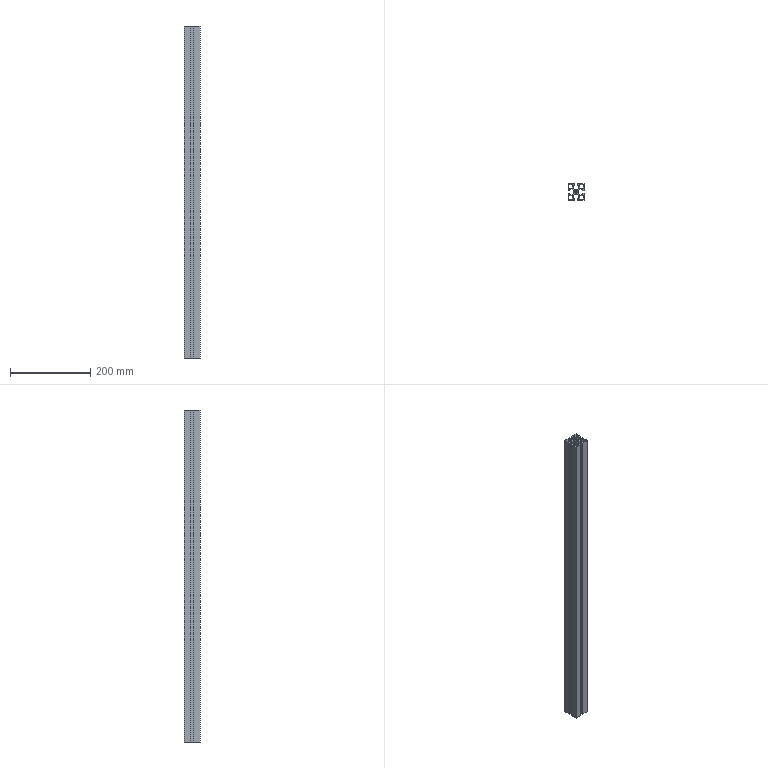Part | STEP file | 40_40_750_1-2 | 1 solid | 64 faces | box 40 x 40 x 830 mm | volume 435537 mm3 | plane 62 | cylinder 2 | commonest cylinder face diameters 6.8 x2